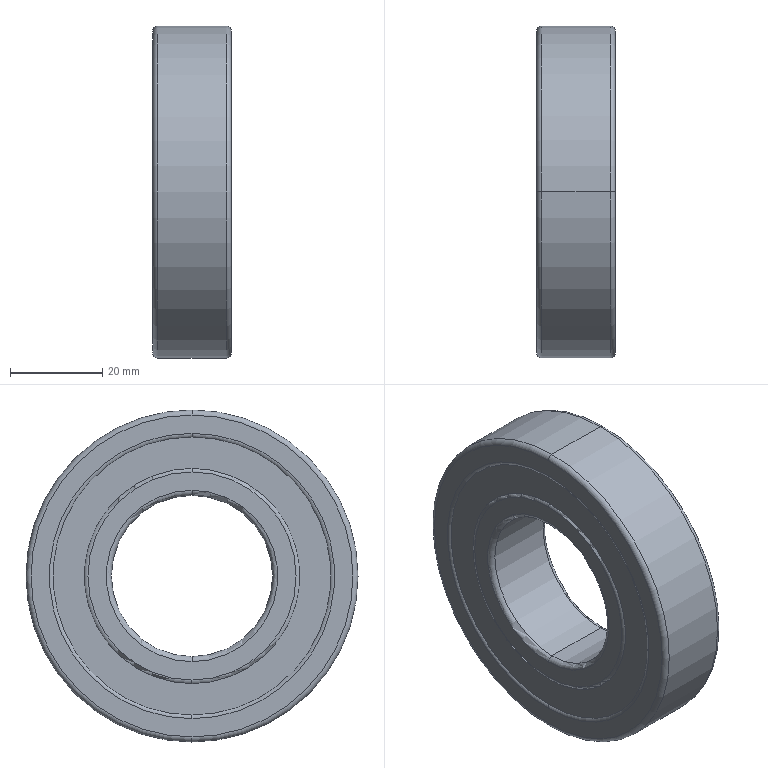Part | SolidWorks | features Revolution 5, CirPattern 2, RefAxis 1, RevCut 1 | 17 solids | 194 faces | box 17 x 72 x 72 mm | volume 40403 mm3 | cylinder 70 | sphere 64 | plane 36 | torus 24 | commonest cylinder face diameters 51.65 x29 55.35 x29 47.333 x4 59.667 x4 35 x2 72 x2